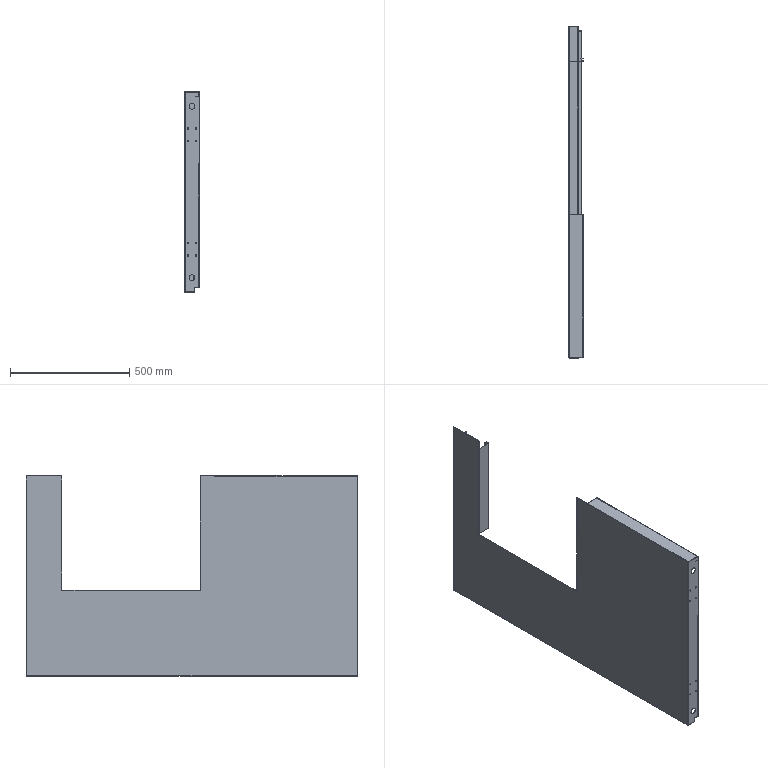Part | SolidWorks | features EdgeFlange 6, ICE 3, FlatPattern 1, SMBaseFlange 1, SheetMetal 1 | 1 solid | 164 faces | box 60 x 1390 x 840 mm | volume 1424848 mm3 | plane 109 | cylinder 49 | spline 6 | commonest cylinder face diameters 5 x16 0.9 x15 3.3 x14 25 x4